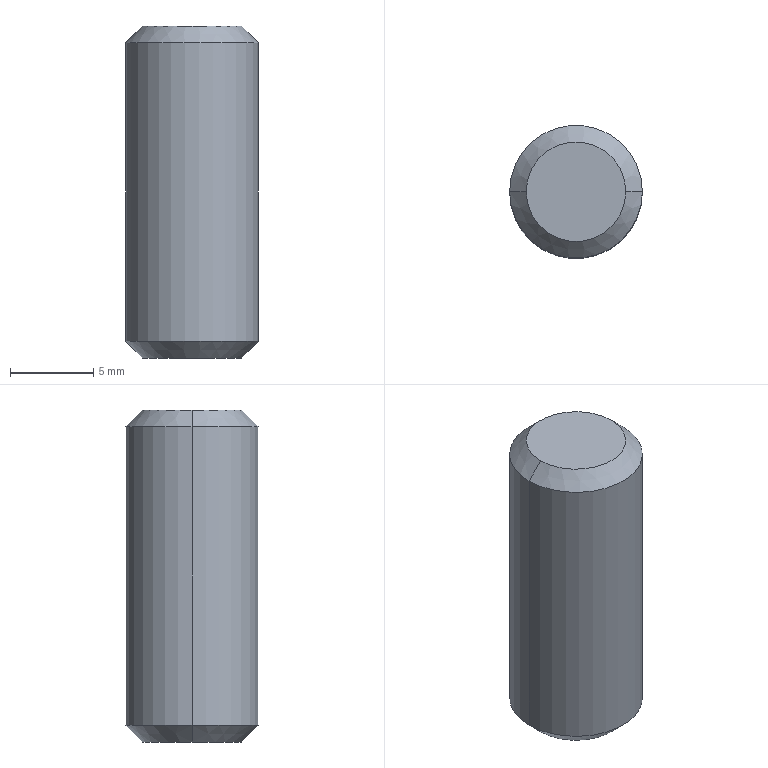Part | SolidWorks | features Chamfer 1, Extrusion 1 | 1 solid | 8 faces | box 8 x 8 x 20 mm | volume 982.271 mm3 | cone 4 | cylinder 2 | plane 2 | commonest cylinder face diameters 8 x2
STEP:
#1=CARTESIAN_POINT('',(3.,0.,20.));
#2=VERTEX_POINT('',#1);
#3=CARTESIAN_POINT('',(-3.,0.,20.));
#4=VERTEX_POINT('',#3);
#5=CARTESIAN_POINT('',(0.,0.,20.));
#6=DIRECTION('',(0.,0.,1.));
#7=DIRECTION('',(1.,0.,0.));
#8=AXIS2_PLACEMENT_3D('',#5,#6,#7);
#9=CIRCLE('',#8,3.);
#10=EDGE_CURVE('',#2,#4,#9,.T.);
#11=ORIENTED_EDGE('',*,*,#10,.F.);
#12=CARTESIAN_POINT('',(4.,0.,19.));
#13=VERTEX_POINT('',#12);
#14=CARTESIAN_POINT('',(3.,0.,20.));
#15=DIRECTION('',(0.7071,0.,-0.7071));
#16=VECTOR('',#15,1000.);
#17=LINE('',#14,#16);
#18=EDGE_CURVE('',#2,#13,#17,.T.);
#19=ORIENTED_EDGE('',*,*,#18,.T.);
#20=CARTESIAN_POINT('',(-4.,0.,19.));
#21=VERTEX_POINT('',#20);
#22=CARTESIAN_POINT('',(0.,0.,19.));
#23=DIRECTION('',(0.,0.,-1.));
#24=DIRECTION('',(1.,0.,0.));
#25=AXIS2_PLACEMENT_3D('',#22,#23,#24);
#26=CIRCLE('',#25,4.);
#27=EDGE_CURVE('',#21,#13,#26,.T.);
#28=ORIENTED_EDGE('',*,*,#27,.F.);
#29=CARTESIAN_POINT('',(-3.,0.,20.));
#30=DIRECTION('',(-0.7071,0.,-0.7071));
#31=VECTOR('',#30,1000.);
#32=LINE('',#29,#31);
#33=EDGE_CURVE('',#4,#21,#32,.T.);
#34=ORIENTED_EDGE('',*,*,#33,.F.);
#35=EDGE_LOOP('',(#11,#19,#28,#34));
#36=FACE_OUTER_BOUND('',#35,.T.);
#37=CARTESIAN_POINT('',(0.,0.,20.));
#38=DIRECTION('',(0.,0.,-1.));
#39=DIRECTION('',(-1.,0.,0.));
#40=AXIS2_PLACEMENT_3D('',#37,#38,#39);
#41=CONICAL_SURFACE('',#40,3.,0.7854);
#42=ADVANCED_FACE('',(#36),#41,.T.);
#43=CARTESIAN_POINT('',(-3.,0.,0.));
#44=VERTEX_POINT('',#43);
#45=CARTESIAN_POINT('',(3.,0.,0.));
#46=VERTEX_POINT('',#45);
#47=CARTESIAN_POINT('',(0.,0.,0.));
#48=DIRECTION('',(0.,0.,-1.));
#49=DIRECTION('',(1.,0.,0.));
#50=AXIS2_PLACEMENT_3D('',#47,#48,#49);
#51=CIRCLE('',#50,3.);
#52=EDGE_CURVE('',#44,#46,#51,.T.);
#53=ORIENTED_EDGE('',*,*,#52,.F.);
#54=CARTESIAN_POINT('',(-4.,0.,1.));
#55=VERTEX_POINT('',#54);
#56=CARTESIAN_POINT('',(-4.,0.,1.));
#57=DIRECTION('',(-0.7071,0.,0.7071));
#58=VECTOR('',#57,1000.);
#59=LINE('',#56,#58);
#60=EDGE_CURVE('',#44,#55,#59,.T.);
#61=ORIENTED_EDGE('',*,*,#60,.T.);
#62=CARTESIAN_POINT('',(4.,0.,1.));
#63=VERTEX_POINT('',#62);
#64=CARTESIAN_POINT('',(0.,0.,1.));
#65=DIRECTION('',(0.,0.,1.));
#66=DIRECTION('',(1.,0.,0.));
#67=AXIS2_PLACEMENT_3D('',#64,#65,#66);
#68=CIRCLE('',#67,4.);
#69=EDGE_CURVE('',#63,#55,#68,.T.);
#70=ORIENTED_EDGE('',*,*,#69,.F.);
#71=CARTESIAN_POINT('',(4.,0.,1.));
#72=DIRECTION('',(0.7071,0.,0.7071));
#73=VECTOR('',#72,1000.);
#74=LINE('',#71,#73);
#75=EDGE_CURVE('',#46,#63,#74,.T.);
#76=ORIENTED_EDGE('',*,*,#75,.F.);
#77=EDGE_LOOP('',(#53,#61,#70,#76));
#78=FACE_OUTER_BOUND('',#77,.T.);
#79=CARTESIAN_POINT('',(0.,0.,1.));
#80=DIRECTION('',(0.,0.,1.));
#81=DIRECTION('',(1.,0.,0.));
#82=AXIS2_PLACEMENT_3D('',#79,#80,#81);
#83=CONICAL_SURFACE('',#82,4.,0.7854);
#84=ADVANCED_FACE('',(#78),#83,.T.);
#85=ORIENTED_EDGE('',*,*,#27,.T.);
#86=CARTESIAN_POINT('',(4.,0.,20.));
#87=DIRECTION('',(0.,0.,-1.));
#88=VECTOR('',#87,1000.);
#89=LINE('',#86,#88);
#90=EDGE_CURVE('',#13,#63,#89,.T.);
#91=ORIENTED_EDGE('',*,*,#90,.T.);
#92=ORIENTED_EDGE('',*,*,#69,.T.);
#93=CARTESIAN_POINT('',(-4.,0.,20.));
#94=DIRECTION('',(0.,0.,-1.));
#95=VECTOR('',#94,1000.);
#96=LINE('',#93,#95);
#97=EDGE_CURVE('',#21,#55,#96,.T.);
#98=ORIENTED_EDGE('',*,*,#97,.F.);
#99=EDGE_LOOP('',(#85,#91,#92,#98));
#100=FACE_OUTER_BOUND('',#99,.T.);
#101=CARTESIAN_POINT('',(0.,0.,20.));
#102=DIRECTION('',(0.,0.,-1.));
#103=DIRECTION('',(-1.,0.,0.));
#104=AXIS2_PLACEMENT_3D('',#101,#102,#103);
#105=CYLINDRICAL_SURFACE('',#104,4.);
#106=ADVANCED_FACE('',(#100),#105,.T.);
#107=ORIENTED_EDGE('',*,*,#90,.F.);
#108=CARTESIAN_POINT('',(0.,0.,19.));
#109=DIRECTION('',(0.,0.,-1.));
#110=DIRECTION('',(1.,0.,0.));
#111=AXIS2_PLACEMENT_3D('',#108,#109,#110);
#112=CIRCLE('',#111,4.);
#113=EDGE_CURVE('',#13,#21,#112,.T.);
#114=ORIENTED_EDGE('',*,*,#113,.T.);
#115=ORIENTED_EDGE('',*,*,#97,.T.);
#116=CARTESIAN_POINT('',(0.,0.,1.));
#117=DIRECTION('',(0.,0.,1.));
#118=DIRECTION('',(1.,0.,0.));
#119=AXIS2_PLACEMENT_3D('',#116,#117,#118);
#120=CIRCLE('',#119,4.);
#121=EDGE_CURVE('',#55,#63,#120,.T.);
#122=ORIENTED_EDGE('',*,*,#121,.T.);
#123=EDGE_LOOP('',(#107,#114,#115,#122));
#124=FACE_OUTER_BOUND('',#123,.T.);
#125=CARTESIAN_POINT('',(0.,0.,20.));
#126=DIRECTION('',(0.,0.,-1.));
#127=DIRECTION('',(-1.,0.,0.));
#128=AXIS2_PLACEMENT_3D('',#125,#126,#127);
#129=CYLINDRICAL_SURFACE('',#128,4.);
#130=ADVANCED_FACE('',(#124),#129,.T.);
#131=CARTESIAN_POINT('',(0.,0.,20.));
#132=DIRECTION('',(0.,0.,1.));
#133=DIRECTION('',(1.,0.,0.));
#134=AXIS2_PLACEMENT_3D('',#131,#132,#133);
#135=CIRCLE('',#134,3.);
#136=EDGE_CURVE('',#4,#2,#135,.T.);
#137=ORIENTED_EDGE('',*,*,#136,.T.);
#138=ORIENTED_EDGE('',*,*,#10,.T.);
#139=EDGE_LOOP('',(#137,#138));
#140=FACE_OUTER_BOUND('',#139,.T.);
#141=CARTESIAN_POINT('',(0.,0.,20.));
#142=DIRECTION('',(0.,0.,1.));
#143=DIRECTION('',(1.,0.,0.));
#144=AXIS2_PLACEMENT_3D('',#141,#142,#143);
#145=PLANE('',#144);
#146=ADVANCED_FACE('',(#140),#145,.T.);
#147=CARTESIAN_POINT('',(0.,0.,0.));
#148=DIRECTION('',(0.,0.,-1.));
#149=DIRECTION('',(1.,0.,0.));
#150=AXIS2_PLACEMENT_3D('',#147,#148,#149);
#151=CIRCLE('',#150,3.);
#152=EDGE_CURVE('',#46,#44,#151,.T.);
#153=ORIENTED_EDGE('',*,*,#152,.T.);
#154=ORIENTED_EDGE('',*,*,#52,.T.);
#155=EDGE_LOOP('',(#153,#154));
#156=FACE_OUTER_BOUND('',#155,.T.);
#157=CARTESIAN_POINT('',(0.,0.,0.));
#158=DIRECTION('',(0.,0.,1.));
#159=DIRECTION('',(1.,0.,0.));
#160=AXIS2_PLACEMENT_3D('',#157,#158,#159);
#161=PLANE('',#160);
#162=ADVANCED_FACE('',(#156),#161,.F.);
#163=ORIENTED_EDGE('',*,*,#60,.F.);
#164=ORIENTED_EDGE('',*,*,#152,.F.);
#165=ORIENTED_EDGE('',*,*,#75,.T.);
#166=ORIENTED_EDGE('',*,*,#121,.F.);
#167=EDGE_LOOP('',(#163,#164,#165,#166));
#168=FACE_OUTER_BOUND('',#167,.T.);
#169=CARTESIAN_POINT('',(0.,0.,1.));
#170=DIRECTION('',(0.,0.,1.));
#171=DIRECTION('',(1.,0.,0.));
#172=AXIS2_PLACEMENT_3D('',#169,#170,#171);
#173=CONICAL_SURFACE('',#172,4.,0.7854);
#174=ADVANCED_FACE('',(#168),#173,.T.);
#175=ORIENTED_EDGE('',*,*,#18,.F.);
#176=ORIENTED_EDGE('',*,*,#136,.F.);
#177=ORIENTED_EDGE('',*,*,#33,.T.);
#178=ORIENTED_EDGE('',*,*,#113,.F.);
#179=EDGE_LOOP('',(#175,#176,#177,#178));
#180=FACE_OUTER_BOUND('',#179,.T.);
#181=CARTESIAN_POINT('',(0.,0.,20.));
#182=DIRECTION('',(0.,0.,-1.));
#183=DIRECTION('',(-1.,0.,0.));
#184=AXIS2_PLACEMENT_3D('',#181,#182,#183);
#185=CONICAL_SURFACE('',#184,3.,0.7854);
#186=ADVANCED_FACE('',(#180),#185,.T.);
#187=CLOSED_SHELL('',(#42,#84,#106,#130,#146,#162,#174,#186));
#188=MANIFOLD_SOLID_BREP('',#187);
#189=CARTESIAN_POINT('',(0.,0.,0.));
#190=DIRECTION('',(0.,0.,1.));
#191=DIRECTION('',(1.,0.,0.));
#192=AXIS2_PLACEMENT_3D('',#189,#190,#191);
#193=(LENGTH_UNIT()NAMED_UNIT(*)SI_UNIT(.MILLI.,.METRE.));
#194=UNCERTAINTY_MEASURE_WITH_UNIT(LENGTH_MEASURE(0.00001),#193,'','');
#195=(NAMED_UNIT(*)PLANE_ANGLE_UNIT()SI_UNIT($,.RADIAN.));
#196=(NAMED_UNIT(*)SI_UNIT($,.STERADIAN.)SOLID_ANGLE_UNIT());
#197=(GEOMETRIC_REPRESENTATION_CONTEXT(3)GLOBAL_UNCERTAINTY_ASSIGNED_CONTEXT((#194))GLOBAL_UNIT_ASSIGNED_CONTEXT((#193,#195,#196))REPRESENTATION_CONTEXT('',''));
#198=ADVANCED_BREP_SHAPE_REPRESENTATION('',(#188,#192),#197);